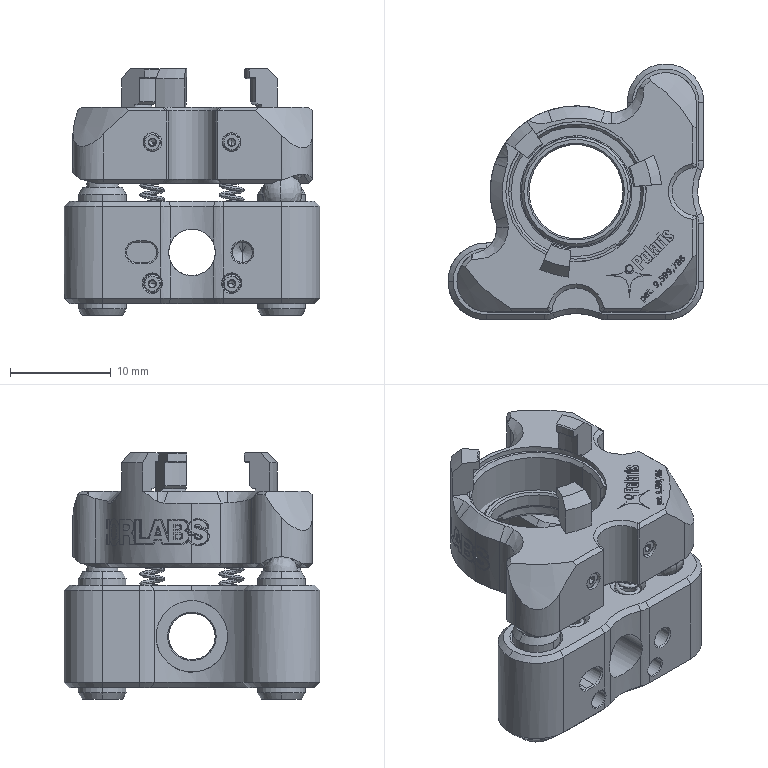Part | SolidWorks | features BaseBody 27 | 26 solids | 2109 faces | box 25.4 x 25.4 x 24.471 mm | volume 4593 mm3 | cone 736 | cylinder 597 | plane 458 | spline 318 | commonest cylinder face diameters 1.854 x221 1.581 x216 0.406 x16 1.511 x16 17.018 x16 2.489 x12